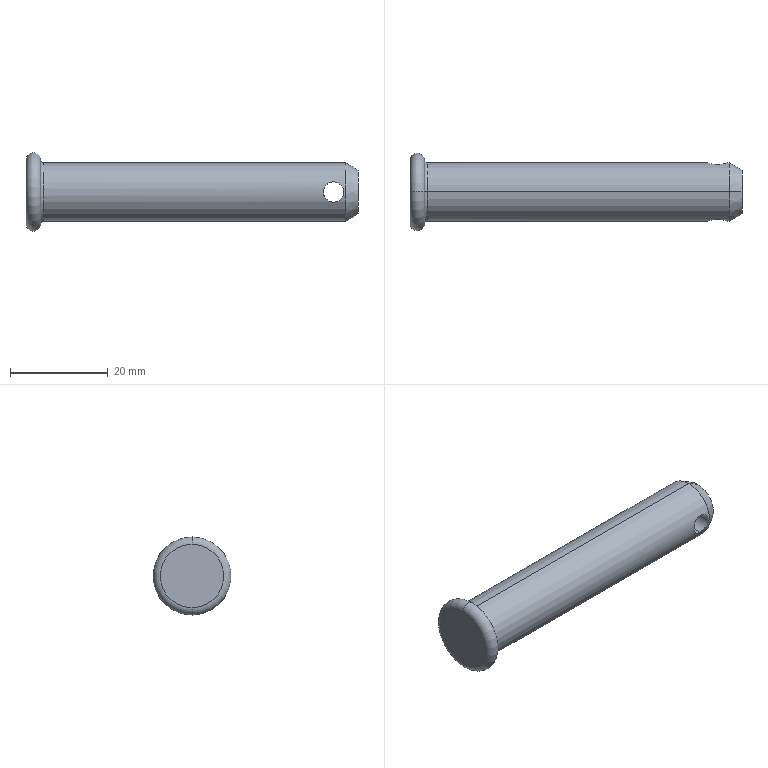Part | STEP file | 1 solid | 12 faces | box 68 x 16 x 16 mm | volume 7681 mm3 | cylinder 4 | torus 4 | cone 2 | plane 2 | commonest cylinder face diameters 4.18 x2 12 x2